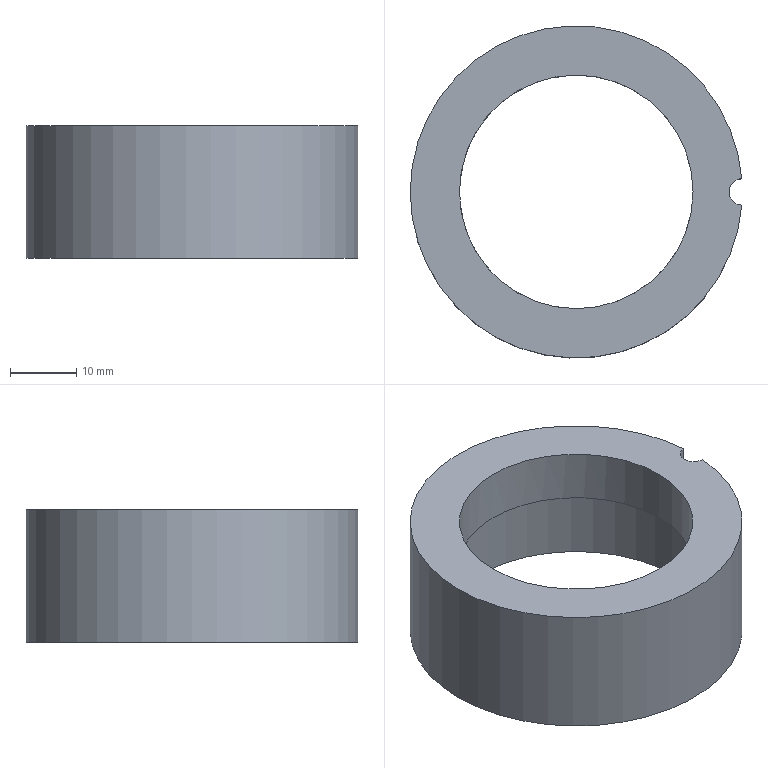Part | NX | features solid 2 | 1 solid | 7 faces | box 49.92 x 50 x 20 mm | volume 15531 mm3 | cylinder 4 | plane 3 | commonest cylinder face diameters 4 x1 35.17 x1 41 x1 50 x1
STEP:
#1=CARTESIAN_POINT('',(-87.149,-93.789,60.815));
#2=VERTEX_POINT('',#1);
#3=CARTESIAN_POINT('',(-87.149,-89.792,60.815));
#4=VERTEX_POINT('',#3);
#5=CARTESIAN_POINT('',(-87.069,-91.791,60.815));
#6=DIRECTION('',(0.,0.,-1.));
#7=DIRECTION('',(-1.,0.,0.));
#8=AXIS2_PLACEMENT_3D('',#5,#6,#7);
#9=CIRCLE('',#8,2.);
#10=EDGE_CURVE('',#2,#4,#9,.T.);
#11=ORIENTED_EDGE('',*,*,#10,.T.);
#12=CARTESIAN_POINT('',(-112.069,-91.791,60.815));
#13=DIRECTION('',(0.,0.,-1.));
#14=DIRECTION('',(-1.,0.,0.));
#15=AXIS2_PLACEMENT_3D('',#12,#13,#14);
#16=CIRCLE('',#15,25.);
#17=EDGE_CURVE('',#2,#4,#16,.T.);
#18=ORIENTED_EDGE('',*,*,#17,.F.);
#19=EDGE_LOOP('',(#11,#18));
#20=FACE_BOUND('',#19,.T.);
#21=CARTESIAN_POINT('',(-129.654,-91.791,60.815));
#22=VERTEX_POINT('',#21);
#23=CARTESIAN_POINT('',(-112.069,-91.791,60.815));
#24=DIRECTION('',(0.,0.,-1.));
#25=DIRECTION('',(-1.,0.,0.));
#26=AXIS2_PLACEMENT_3D('',#23,#24,#25);
#27=CIRCLE('',#26,17.585);
#28=EDGE_CURVE('',#22,#22,#27,.T.);
#29=ORIENTED_EDGE('',*,*,#28,.T.);
#30=EDGE_LOOP('',(#29));
#31=FACE_BOUND('',#30,.T.);
#32=CARTESIAN_POINT('',(-112.069,-91.791,60.815));
#33=DIRECTION('',(0.,0.,1.));
#34=DIRECTION('',(1.,0.,0.));
#35=AXIS2_PLACEMENT_3D('',#32,#33,#34);
#36=PLANE('',#35);
#37=ADVANCED_FACE('',(#20,#31),#36,.T.);
#38=CARTESIAN_POINT('',(-87.149,-89.792,40.815));
#39=VERTEX_POINT('',#38);
#40=CARTESIAN_POINT('',(-87.149,-93.789,40.815));
#41=VERTEX_POINT('',#40);
#42=CARTESIAN_POINT('',(-87.069,-91.791,40.815));
#43=DIRECTION('',(0.,0.,1.));
#44=DIRECTION('',(1.,0.,0.));
#45=AXIS2_PLACEMENT_3D('',#42,#43,#44);
#46=CIRCLE('',#45,2.);
#47=EDGE_CURVE('',#39,#41,#46,.T.);
#48=ORIENTED_EDGE('',*,*,#47,.T.);
#49=CARTESIAN_POINT('',(-112.069,-91.791,40.815));
#50=DIRECTION('',(0.,0.,1.));
#51=DIRECTION('',(1.,0.,0.));
#52=AXIS2_PLACEMENT_3D('',#49,#50,#51);
#53=CIRCLE('',#52,25.);
#54=EDGE_CURVE('',#39,#41,#53,.T.);
#55=ORIENTED_EDGE('',*,*,#54,.F.);
#56=EDGE_LOOP('',(#48,#55));
#57=FACE_BOUND('',#56,.T.);
#58=CARTESIAN_POINT('',(-91.569,-91.791,40.815));
#59=VERTEX_POINT('',#58);
#60=CARTESIAN_POINT('',(-112.069,-91.791,40.815));
#61=DIRECTION('',(0.,0.,1.));
#62=DIRECTION('',(1.,0.,0.));
#63=AXIS2_PLACEMENT_3D('',#60,#61,#62);
#64=CIRCLE('',#63,20.5);
#65=EDGE_CURVE('',#59,#59,#64,.T.);
#66=ORIENTED_EDGE('',*,*,#65,.T.);
#67=EDGE_LOOP('',(#66));
#68=FACE_BOUND('',#67,.T.);
#69=CARTESIAN_POINT('',(-112.069,-91.791,40.815));
#70=DIRECTION('',(0.,0.,-1.));
#71=DIRECTION('',(-1.,0.,0.));
#72=AXIS2_PLACEMENT_3D('',#69,#70,#71);
#73=PLANE('',#72);
#74=ADVANCED_FACE('',(#57,#68),#73,.T.);
#75=CARTESIAN_POINT('',(-87.149,-89.792,50.815));
#76=DIRECTION('',(0.,0.,1.));
#77=VECTOR('',#76,1000.);
#78=LINE('',#75,#77);
#79=EDGE_CURVE('',#39,#4,#78,.T.);
#80=ORIENTED_EDGE('',*,*,#79,.F.);
#81=ORIENTED_EDGE('',*,*,#54,.T.);
#82=CARTESIAN_POINT('',(-87.149,-93.789,50.815));
#83=DIRECTION('',(0.,0.,1.));
#84=VECTOR('',#83,1000.);
#85=LINE('',#82,#84);
#86=EDGE_CURVE('',#2,#41,#85,.F.);
#87=ORIENTED_EDGE('',*,*,#86,.F.);
#88=ORIENTED_EDGE('',*,*,#17,.T.);
#89=EDGE_LOOP('',(#80,#81,#87,#88));
#90=FACE_BOUND('',#89,.T.);
#91=CARTESIAN_POINT('',(-112.069,-91.791,40.815));
#92=DIRECTION('',(0.,0.,1.));
#93=DIRECTION('',(1.,0.,0.));
#94=AXIS2_PLACEMENT_3D('',#91,#92,#93);
#95=CYLINDRICAL_SURFACE('',#94,25.);
#96=ADVANCED_FACE('',(#90),#95,.T.);
#97=CARTESIAN_POINT('',(-94.484,-91.791,52.815));
#98=VERTEX_POINT('',#97);
#99=CARTESIAN_POINT('',(-112.069,-91.791,52.815));
#100=DIRECTION('',(0.,0.,1.));
#101=DIRECTION('',(1.,0.,0.));
#102=AXIS2_PLACEMENT_3D('',#99,#100,#101);
#103=CIRCLE('',#102,17.585);
#104=EDGE_CURVE('',#98,#98,#103,.T.);
#105=ORIENTED_EDGE('',*,*,#104,.T.);
#106=EDGE_LOOP('',(#105));
#107=FACE_BOUND('',#106,.T.);
#108=CARTESIAN_POINT('',(-132.569,-91.791,52.815));
#109=VERTEX_POINT('',#108);
#110=CARTESIAN_POINT('',(-112.069,-91.791,52.815));
#111=DIRECTION('',(0.,0.,-1.));
#112=DIRECTION('',(-1.,0.,0.));
#113=AXIS2_PLACEMENT_3D('',#110,#111,#112);
#114=CIRCLE('',#113,20.5);
#115=EDGE_CURVE('',#109,#109,#114,.T.);
#116=ORIENTED_EDGE('',*,*,#115,.T.);
#117=EDGE_LOOP('',(#116));
#118=FACE_BOUND('',#117,.T.);
#119=CARTESIAN_POINT('',(-112.069,-91.791,52.815));
#120=DIRECTION('',(0.,0.,1.));
#121=DIRECTION('',(1.,0.,0.));
#122=AXIS2_PLACEMENT_3D('',#119,#120,#121);
#123=PLANE('',#122);
#124=ADVANCED_FACE('',(#107,#118),#123,.F.);
#125=ORIENTED_EDGE('',*,*,#115,.F.);
#126=EDGE_LOOP('',(#125));
#127=FACE_BOUND('',#126,.T.);
#128=ORIENTED_EDGE('',*,*,#65,.F.);
#129=EDGE_LOOP('',(#128));
#130=FACE_BOUND('',#129,.T.);
#131=CARTESIAN_POINT('',(-112.069,-91.791,40.815));
#132=DIRECTION('',(0.,0.,1.));
#133=DIRECTION('',(1.,0.,0.));
#134=AXIS2_PLACEMENT_3D('',#131,#132,#133);
#135=CYLINDRICAL_SURFACE('',#134,20.5);
#136=ADVANCED_FACE('',(#127,#130),#135,.F.);
#137=ORIENTED_EDGE('',*,*,#28,.F.);
#138=EDGE_LOOP('',(#137));
#139=FACE_BOUND('',#138,.T.);
#140=ORIENTED_EDGE('',*,*,#104,.F.);
#141=EDGE_LOOP('',(#140));
#142=FACE_BOUND('',#141,.T.);
#143=CARTESIAN_POINT('',(-112.069,-91.791,52.815));
#144=DIRECTION('',(0.,0.,1.));
#145=DIRECTION('',(1.,0.,0.));
#146=AXIS2_PLACEMENT_3D('',#143,#144,#145);
#147=CYLINDRICAL_SURFACE('',#146,17.585);
#148=ADVANCED_FACE('',(#139,#142),#147,.F.);
#149=ORIENTED_EDGE('',*,*,#79,.T.);
#150=ORIENTED_EDGE('',*,*,#10,.F.);
#151=ORIENTED_EDGE('',*,*,#86,.T.);
#152=ORIENTED_EDGE('',*,*,#47,.F.);
#153=EDGE_LOOP('',(#149,#150,#151,#152));
#154=FACE_BOUND('',#153,.T.);
#155=CARTESIAN_POINT('',(-87.069,-91.791,40.815));
#156=DIRECTION('',(0.,0.,1.));
#157=DIRECTION('',(1.,0.,0.));
#158=AXIS2_PLACEMENT_3D('',#155,#156,#157);
#159=CYLINDRICAL_SURFACE('',#158,2.);
#160=ADVANCED_FACE('',(#154),#159,.F.);
#161=CLOSED_SHELL('',(#37,#74,#96,#124,#136,#148,#160));
#162=MANIFOLD_SOLID_BREP('',#161);
#163=(LENGTH_UNIT()NAMED_UNIT(*)SI_UNIT(.MILLI.,.METRE.));
#164=UNCERTAINTY_MEASURE_WITH_UNIT(LENGTH_MEASURE(0.00001),#163,'','');
#165=(NAMED_UNIT(*)PLANE_ANGLE_UNIT()SI_UNIT($,.RADIAN.));
#166=(NAMED_UNIT(*)SI_UNIT($,.STERADIAN.)SOLID_ANGLE_UNIT());
#167=(GEOMETRIC_REPRESENTATION_CONTEXT(3)GLOBAL_UNCERTAINTY_ASSIGNED_CONTEXT((#164))GLOBAL_UNIT_ASSIGNED_CONTEXT((#163,#165,#166))REPRESENTATION_CONTEXT('',''));
#168=ADVANCED_BREP_SHAPE_REPRESENTATION('',(#162),#167);